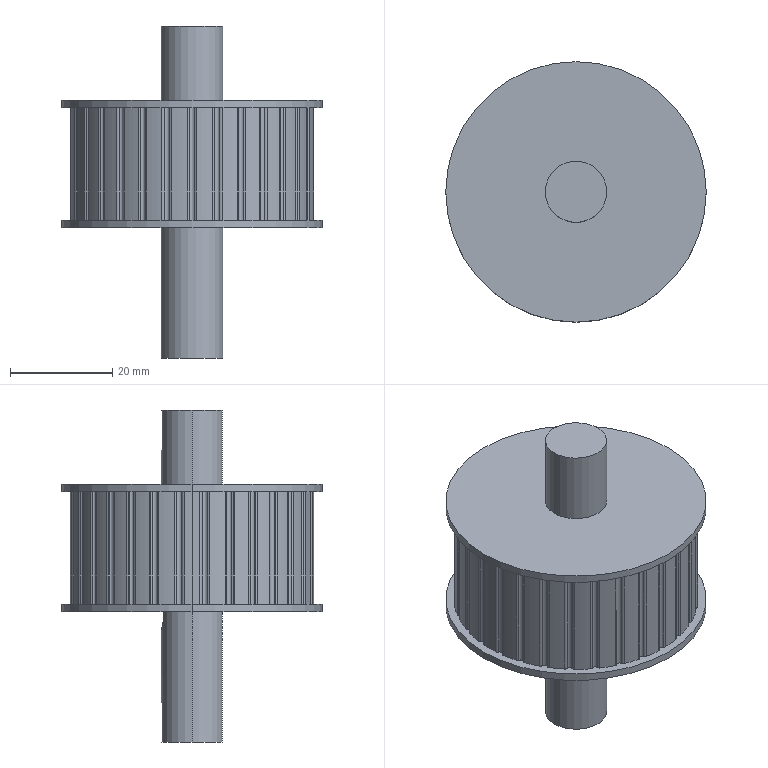Part | 2 solids | 161 faces | box 51 x 51 x 65 mm | volume 49533 mm3 | cylinder 152 | plane 9 | commonest cylinder face diameters 0.96 x70 1.14 x40 47.75 x31 12 x4 51 x4 4 x3